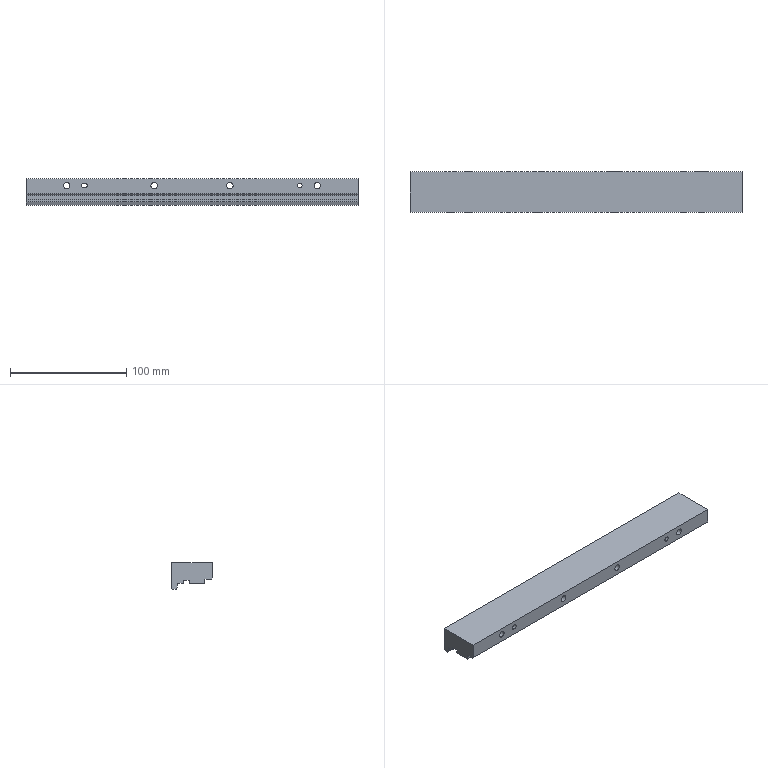Part | NX | 1 solid | 35 faces | box 285 x 35 x 22.9 mm | volume 168011 mm3 | plane 24 | cylinder 11 | commonest cylinder face diameters 5.5 x4 10 x4 4 x3
STEP:
#1=CARTESIAN_POINT('',(142.5,-17.5,-13.1));
#2=VERTEX_POINT('',#1);
#3=CARTESIAN_POINT('',(142.5,-16.5,-14.1));
#4=VERTEX_POINT('',#3);
#5=CARTESIAN_POINT('',(142.5,-17.5,-13.1));
#6=DIRECTION('',(0.,0.7071,-0.7071));
#7=VECTOR('',#6,1000.);
#8=LINE('',#5,#7);
#9=EDGE_CURVE('',#2,#4,#8,.T.);
#10=ORIENTED_EDGE('',*,*,#9,.T.);
#11=CARTESIAN_POINT('',(142.5,-11.14,-14.1));
#12=VERTEX_POINT('',#11);
#13=CARTESIAN_POINT('',(142.5,-17.5,-14.1));
#14=DIRECTION('',(0.,-1.,0.));
#15=VECTOR('',#14,1000.);
#16=LINE('',#13,#15);
#17=EDGE_CURVE('',#12,#4,#16,.T.);
#18=ORIENTED_EDGE('',*,*,#17,.F.);
#19=CARTESIAN_POINT('',(142.5,-11.14,-17.9));
#20=VERTEX_POINT('',#19);
#21=CARTESIAN_POINT('',(142.5,-11.14,-14.1));
#22=DIRECTION('',(0.,0.,1.));
#23=VECTOR('',#22,1000.);
#24=LINE('',#21,#23);
#25=EDGE_CURVE('',#20,#12,#24,.T.);
#26=ORIENTED_EDGE('',*,*,#25,.F.);
#27=CARTESIAN_POINT('',(142.5,2.3,-17.9));
#28=VERTEX_POINT('',#27);
#29=CARTESIAN_POINT('',(142.5,17.5,-17.9));
#30=DIRECTION('',(0.,-1.,0.));
#31=VECTOR('',#30,1000.);
#32=LINE('',#29,#31);
#33=EDGE_CURVE('',#28,#20,#32,.T.);
#34=ORIENTED_EDGE('',*,*,#33,.F.);
#35=CARTESIAN_POINT('',(142.5,2.3,-14.9));
#36=VERTEX_POINT('',#35);
#37=CARTESIAN_POINT('',(142.5,2.3,-17.9));
#38=DIRECTION('',(0.,0.,-1.));
#39=VECTOR('',#38,1000.);
#40=LINE('',#37,#39);
#41=EDGE_CURVE('',#36,#28,#40,.T.);
#42=ORIENTED_EDGE('',*,*,#41,.F.);
#43=CARTESIAN_POINT('',(142.5,7.3,-14.9));
#44=VERTEX_POINT('',#43);
#45=CARTESIAN_POINT('',(142.5,2.3,-14.9));
#46=DIRECTION('',(0.,-1.,0.));
#47=VECTOR('',#46,1000.);
#48=LINE('',#45,#47);
#49=EDGE_CURVE('',#44,#36,#48,.T.);
#50=ORIENTED_EDGE('',*,*,#49,.F.);
#51=CARTESIAN_POINT('',(142.5,7.3,-17.04));
#52=VERTEX_POINT('',#51);
#53=CARTESIAN_POINT('',(142.5,7.3,-14.9));
#54=DIRECTION('',(0.,0.,1.));
#55=VECTOR('',#54,1000.);
#56=LINE('',#53,#55);
#57=EDGE_CURVE('',#52,#44,#56,.T.);
#58=ORIENTED_EDGE('',*,*,#57,.F.);
#59=CARTESIAN_POINT('',(142.5,7.533,-17.54));
#60=VERTEX_POINT('',#59);
#61=CARTESIAN_POINT('',(142.5,7.3,-17.04));
#62=DIRECTION('',(0.,0.4226,-0.9063));
#63=VECTOR('',#62,1000.);
#64=LINE('',#61,#63);
#65=EDGE_CURVE('',#52,#60,#64,.T.);
#66=ORIENTED_EDGE('',*,*,#65,.T.);
#67=CARTESIAN_POINT('',(142.5,12.2,-17.54));
#68=VERTEX_POINT('',#67);
#69=CARTESIAN_POINT('',(142.5,7.3,-17.54));
#70=DIRECTION('',(0.,-1.,0.));
#71=VECTOR('',#70,1000.);
#72=LINE('',#69,#71);
#73=EDGE_CURVE('',#68,#60,#72,.T.);
#74=ORIENTED_EDGE('',*,*,#73,.F.);
#75=CARTESIAN_POINT('',(142.5,12.2,-19.9));
#76=VERTEX_POINT('',#75);
#77=CARTESIAN_POINT('',(142.5,12.2,-17.54));
#78=DIRECTION('',(0.,0.,1.));
#79=VECTOR('',#78,1000.);
#80=LINE('',#77,#79);
#81=EDGE_CURVE('',#76,#68,#80,.T.);
#82=ORIENTED_EDGE('',*,*,#81,.F.);
#83=CARTESIAN_POINT('',(142.5,13.599,-22.9));
#84=VERTEX_POINT('',#83);
#85=CARTESIAN_POINT('',(142.5,13.599,-22.9));
#86=DIRECTION('',(0.,0.4226,-0.9063));
#87=VECTOR('',#86,1000.);
#88=LINE('',#85,#87);
#89=EDGE_CURVE('',#76,#84,#88,.T.);
#90=ORIENTED_EDGE('',*,*,#89,.T.);
#91=CARTESIAN_POINT('',(142.5,16.5,-22.9));
#92=VERTEX_POINT('',#91);
#93=CARTESIAN_POINT('',(142.5,0.,-22.9));
#94=DIRECTION('',(0.,1.,0.));
#95=VECTOR('',#94,1000.);
#96=LINE('',#93,#95);
#97=EDGE_CURVE('',#84,#92,#96,.T.);
#98=ORIENTED_EDGE('',*,*,#97,.T.);
#99=CARTESIAN_POINT('',(142.5,17.5,-21.9));
#100=VERTEX_POINT('',#99);
#101=CARTESIAN_POINT('',(142.5,16.5,-22.9));
#102=DIRECTION('',(0.,0.7071,0.7071));
#103=VECTOR('',#102,1000.);
#104=LINE('',#101,#103);
#105=EDGE_CURVE('',#92,#100,#104,.T.);
#106=ORIENTED_EDGE('',*,*,#105,.T.);
#107=CARTESIAN_POINT('',(142.5,17.5,0.));
#108=VERTEX_POINT('',#107);
#109=CARTESIAN_POINT('',(142.5,17.5,-17.9));
#110=DIRECTION('',(0.,0.,1.));
#111=VECTOR('',#110,1000.);
#112=LINE('',#109,#111);
#113=EDGE_CURVE('',#100,#108,#112,.T.);
#114=ORIENTED_EDGE('',*,*,#113,.T.);
#115=CARTESIAN_POINT('',(142.5,-17.5,0.));
#116=VERTEX_POINT('',#115);
#117=CARTESIAN_POINT('',(142.5,17.5,0.));
#118=DIRECTION('',(0.,1.,0.));
#119=VECTOR('',#118,1000.);
#120=LINE('',#117,#119);
#121=EDGE_CURVE('',#116,#108,#120,.T.);
#122=ORIENTED_EDGE('',*,*,#121,.F.);
#123=CARTESIAN_POINT('',(142.5,-17.5,-17.9));
#124=DIRECTION('',(0.,0.,1.));
#125=VECTOR('',#124,1000.);
#126=LINE('',#123,#125);
#127=EDGE_CURVE('',#2,#116,#126,.T.);
#128=ORIENTED_EDGE('',*,*,#127,.F.);
#129=EDGE_LOOP('',(#10,#18,#26,#34,#42,#50,#58,#66,#74,#82,#90,#98,#106,#114,#122,#128));
#130=FACE_BOUND('',#129,.T.);
#131=CARTESIAN_POINT('',(142.5,17.5,-22.91));
#132=DIRECTION('',(-1.,0.,0.));
#133=DIRECTION('',(0.,0.,-1.));
#134=AXIS2_PLACEMENT_3D('',#131,#132,#133);
#135=PLANE('',#134);
#136=ADVANCED_FACE('',(#130),#135,.F.);
#137=ORIENTED_EDGE('',*,*,#65,.F.);
#138=CARTESIAN_POINT('',(-142.5,7.3,-17.04));
#139=VERTEX_POINT('',#138);
#140=CARTESIAN_POINT('',(-142.5,7.3,-17.04));
#141=DIRECTION('',(1.,0.,0.));
#142=VECTOR('',#141,1000.);
#143=LINE('',#140,#142);
#144=EDGE_CURVE('',#139,#52,#143,.T.);
#145=ORIENTED_EDGE('',*,*,#144,.F.);
#146=CARTESIAN_POINT('',(-142.5,7.533,-17.54));
#147=VERTEX_POINT('',#146);
#148=CARTESIAN_POINT('',(-142.5,7.3,-17.04));
#149=DIRECTION('',(0.,-0.4226,0.9063));
#150=VECTOR('',#149,1000.);
#151=LINE('',#148,#150);
#152=EDGE_CURVE('',#147,#139,#151,.T.);
#153=ORIENTED_EDGE('',*,*,#152,.F.);
#154=CARTESIAN_POINT('',(-142.5,7.533,-17.54));
#155=DIRECTION('',(-1.,0.,0.));
#156=VECTOR('',#155,1000.);
#157=LINE('',#154,#156);
#158=EDGE_CURVE('',#60,#147,#157,.T.);
#159=ORIENTED_EDGE('',*,*,#158,.F.);
#160=EDGE_LOOP('',(#137,#145,#153,#159));
#161=FACE_BOUND('',#160,.T.);
#162=CARTESIAN_POINT('',(-142.5,7.3,-17.04));
#163=DIRECTION('',(0.,0.9063,0.4226));
#164=DIRECTION('',(-1.,0.,0.));
#165=AXIS2_PLACEMENT_3D('',#162,#163,#164);
#166=PLANE('',#165);
#167=ADVANCED_FACE('',(#161),#166,.F.);
#168=ORIENTED_EDGE('',*,*,#144,.T.);
#169=ORIENTED_EDGE('',*,*,#57,.T.);
#170=CARTESIAN_POINT('',(-142.5,7.3,-14.9));
#171=VERTEX_POINT('',#170);
#172=CARTESIAN_POINT('',(-142.5,7.3,-14.9));
#173=DIRECTION('',(1.,0.,0.));
#174=VECTOR('',#173,1000.);
#175=LINE('',#172,#174);
#176=EDGE_CURVE('',#171,#44,#175,.T.);
#177=ORIENTED_EDGE('',*,*,#176,.F.);
#178=CARTESIAN_POINT('',(-142.5,7.3,-14.9));
#179=DIRECTION('',(0.,0.,1.));
#180=VECTOR('',#179,1000.);
#181=LINE('',#178,#180);
#182=EDGE_CURVE('',#139,#171,#181,.T.);
#183=ORIENTED_EDGE('',*,*,#182,.F.);
#184=EDGE_LOOP('',(#168,#169,#177,#183));
#185=FACE_BOUND('',#184,.T.);
#186=CARTESIAN_POINT('',(-142.5,7.3,-14.9));
#187=DIRECTION('',(0.,1.,0.));
#188=DIRECTION('',(0.,0.,1.));
#189=AXIS2_PLACEMENT_3D('',#186,#187,#188);
#190=PLANE('',#189);
#191=ADVANCED_FACE('',(#185),#190,.F.);
#192=CARTESIAN_POINT('',(-142.5,-11.14,-17.9));
#193=VERTEX_POINT('',#192);
#194=CARTESIAN_POINT('',(-142.5,-11.14,-17.9));
#195=DIRECTION('',(1.,0.,0.));
#196=VECTOR('',#195,1000.);
#197=LINE('',#194,#196);
#198=EDGE_CURVE('',#193,#20,#197,.T.);
#199=ORIENTED_EDGE('',*,*,#198,.T.);
#200=ORIENTED_EDGE('',*,*,#25,.T.);
#201=CARTESIAN_POINT('',(-142.5,-11.14,-14.1));
#202=VERTEX_POINT('',#201);
#203=CARTESIAN_POINT('',(-142.5,-11.14,-14.1));
#204=DIRECTION('',(1.,0.,0.));
#205=VECTOR('',#204,1000.);
#206=LINE('',#203,#205);
#207=EDGE_CURVE('',#202,#12,#206,.T.);
#208=ORIENTED_EDGE('',*,*,#207,.F.);
#209=CARTESIAN_POINT('',(-142.5,-11.14,-14.1));
#210=DIRECTION('',(0.,0.,1.));
#211=VECTOR('',#210,1000.);
#212=LINE('',#209,#211);
#213=EDGE_CURVE('',#193,#202,#212,.T.);
#214=ORIENTED_EDGE('',*,*,#213,.F.);
#215=EDGE_LOOP('',(#199,#200,#208,#214));
#216=FACE_BOUND('',#215,.T.);
#217=CARTESIAN_POINT('',(-142.5,-11.14,-14.1));
#218=DIRECTION('',(0.,1.,0.));
#219=DIRECTION('',(0.,0.,1.));
#220=AXIS2_PLACEMENT_3D('',#217,#218,#219);
#221=PLANE('',#220);
#222=ADVANCED_FACE('',(#216),#221,.F.);
#223=CARTESIAN_POINT('',(-142.5,2.3,-17.9));
#224=VERTEX_POINT('',#223);
#225=CARTESIAN_POINT('',(-142.5,2.3,-17.9));
#226=DIRECTION('',(1.,0.,0.));
#227=VECTOR('',#226,1000.);
#228=LINE('',#225,#227);
#229=EDGE_CURVE('',#224,#28,#228,.T.);
#230=ORIENTED_EDGE('',*,*,#229,.T.);
#231=ORIENTED_EDGE('',*,*,#33,.T.);
#232=ORIENTED_EDGE('',*,*,#198,.F.);
#233=CARTESIAN_POINT('',(-142.5,17.5,-17.9));
#234=DIRECTION('',(0.,-1.,0.));
#235=VECTOR('',#234,1000.);
#236=LINE('',#233,#235);
#237=EDGE_CURVE('',#224,#193,#236,.T.);
#238=ORIENTED_EDGE('',*,*,#237,.F.);
#239=EDGE_LOOP('',(#230,#231,#232,#238));
#240=FACE_BOUND('',#239,.T.);
#241=CARTESIAN_POINT('',(1442.5,17.5,-17.9));
#242=DIRECTION('',(0.,0.,1.));
#243=DIRECTION('',(-1.,0.,0.));
#244=AXIS2_PLACEMENT_3D('',#241,#242,#243);
#245=PLANE('',#244);
#246=ADVANCED_FACE('',(#240),#245,.F.);
#247=ORIENTED_EDGE('',*,*,#9,.F.);
#248=CARTESIAN_POINT('',(-142.5,-17.5,-13.1));
#249=VERTEX_POINT('',#248);
#250=CARTESIAN_POINT('',(1442.5,-17.5,-13.1));
#251=DIRECTION('',(1.,0.,0.));
#252=VECTOR('',#251,1000.);
#253=LINE('',#250,#252);
#254=EDGE_CURVE('',#249,#2,#253,.T.);
#255=ORIENTED_EDGE('',*,*,#254,.F.);
#256=CARTESIAN_POINT('',(-142.5,-16.5,-14.1));
#257=VERTEX_POINT('',#256);
#258=CARTESIAN_POINT('',(-142.5,-17.5,-13.1));
#259=DIRECTION('',(0.,-0.7071,0.7071));
#260=VECTOR('',#259,1000.);
#261=LINE('',#258,#260);
#262=EDGE_CURVE('',#257,#249,#261,.T.);
#263=ORIENTED_EDGE('',*,*,#262,.F.);
#264=CARTESIAN_POINT('',(-142.5,-16.5,-14.1));
#265=DIRECTION('',(-1.,0.,0.));
#266=VECTOR('',#265,1000.);
#267=LINE('',#264,#266);
#268=EDGE_CURVE('',#4,#257,#267,.T.);
#269=ORIENTED_EDGE('',*,*,#268,.F.);
#270=EDGE_LOOP('',(#247,#255,#263,#269));
#271=FACE_BOUND('',#270,.T.);
#272=CARTESIAN_POINT('',(1442.5,-17.5,-13.1));
#273=DIRECTION('',(0.,0.7071,0.7071));
#274=DIRECTION('',(-1.,0.,0.));
#275=AXIS2_PLACEMENT_3D('',#272,#273,#274);
#276=PLANE('',#275);
#277=ADVANCED_FACE('',(#271),#276,.F.);
#278=CARTESIAN_POINT('',(-92.,-17.5,-8.));
#279=VERTEX_POINT('',#278);
#280=CARTESIAN_POINT('',(-93.,-17.5,-8.));
#281=VERTEX_POINT('',#280);
#282=CARTESIAN_POINT('',(-93.,-17.5,-8.));
#283=DIRECTION('',(-1.,0.,0.));
#284=VECTOR('',#283,1000.);
#285=LINE('',#282,#284);
#286=EDGE_CURVE('',#279,#281,#285,.T.);
#287=ORIENTED_EDGE('',*,*,#286,.T.);
#288=CARTESIAN_POINT('',(-93.,-17.5,-4.));
#289=VERTEX_POINT('',#288);
#290=CARTESIAN_POINT('',(-93.,-17.5,-6.));
#291=DIRECTION('',(0.,1.,0.));
#292=DIRECTION('',(0.,0.,-1.));
#293=AXIS2_PLACEMENT_3D('',#290,#291,#292);
#294=CIRCLE('',#293,2.);
#295=EDGE_CURVE('',#281,#289,#294,.T.);
#296=ORIENTED_EDGE('',*,*,#295,.T.);
#297=CARTESIAN_POINT('',(-92.,-17.5,-4.));
#298=VERTEX_POINT('',#297);
#299=CARTESIAN_POINT('',(-93.,-17.5,-4.));
#300=DIRECTION('',(1.,0.,0.));
#301=VECTOR('',#300,1000.);
#302=LINE('',#299,#301);
#303=EDGE_CURVE('',#289,#298,#302,.T.);
#304=ORIENTED_EDGE('',*,*,#303,.T.);
#305=CARTESIAN_POINT('',(-92.,-17.5,-6.));
#306=DIRECTION('',(0.,1.,0.));
#307=DIRECTION('',(0.,0.,-1.));
#308=AXIS2_PLACEMENT_3D('',#305,#306,#307);
#309=CIRCLE('',#308,2.);
#310=EDGE_CURVE('',#298,#279,#309,.T.);
#311=ORIENTED_EDGE('',*,*,#310,.T.);
#312=EDGE_LOOP('',(#287,#296,#304,#311));
#313=FACE_BOUND('',#312,.T.);
#314=CARTESIAN_POINT('',(92.5,-17.5,-8.));
#315=VERTEX_POINT('',#314);
#316=CARTESIAN_POINT('',(92.5,-17.5,-6.));
#317=DIRECTION('',(0.,1.,0.));
#318=DIRECTION('',(0.,0.,-1.));
#319=AXIS2_PLACEMENT_3D('',#316,#317,#318);
#320=CIRCLE('',#319,2.);
#321=EDGE_CURVE('',#315,#315,#320,.T.);
#322=ORIENTED_EDGE('',*,*,#321,.T.);
#323=EDGE_LOOP('',(#322));
#324=FACE_BOUND('',#323,.T.);
#325=CARTESIAN_POINT('',(107.5,-17.5,-8.75));
#326=VERTEX_POINT('',#325);
#327=CARTESIAN_POINT('',(107.5,-17.5,-6.));
#328=DIRECTION('',(0.,1.,0.));
#329=DIRECTION('',(0.,0.,-1.));
#330=AXIS2_PLACEMENT_3D('',#327,#328,#329);
#331=CIRCLE('',#330,2.75);
#332=EDGE_CURVE('',#326,#326,#331,.T.);
#333=ORIENTED_EDGE('',*,*,#332,.T.);
#334=EDGE_LOOP('',(#333));
#335=FACE_BOUND('',#334,.T.);
#336=CARTESIAN_POINT('',(32.5,-17.5,-8.75));
#337=VERTEX_POINT('',#336);
#338=CARTESIAN_POINT('',(32.5,-17.5,-6.));
#339=DIRECTION('',(0.,1.,0.));
#340=DIRECTION('',(0.,0.,-1.));
#341=AXIS2_PLACEMENT_3D('',#338,#339,#340);
#342=CIRCLE('',#341,2.75);
#343=EDGE_CURVE('',#337,#337,#342,.T.);
#344=ORIENTED_EDGE('',*,*,#343,.T.);
#345=EDGE_LOOP('',(#344));
#346=FACE_BOUND('',#345,.T.);
#347=CARTESIAN_POINT('',(-32.5,-17.5,-8.75));
#348=VERTEX_POINT('',#347);
#349=CARTESIAN_POINT('',(-32.5,-17.5,-6.));
#350=DIRECTION('',(0.,1.,0.));
#351=DIRECTION('',(0.,0.,-1.));
#352=AXIS2_PLACEMENT_3D('',#349,#350,#351);
#353=CIRCLE('',#352,2.75);
#354=EDGE_CURVE('',#348,#348,#353,.T.);
#355=ORIENTED_EDGE('',*,*,#354,.T.);
#356=EDGE_LOOP('',(#355));
#357=FACE_BOUND('',#356,.T.);
#358=CARTESIAN_POINT('',(-107.5,-17.5,-8.75));
#359=VERTEX_POINT('',#358);
#360=CARTESIAN_POINT('',(-107.5,-17.5,-6.));
#361=DIRECTION('',(0.,1.,0.));
#362=DIRECTION('',(0.,0.,-1.));
#363=AXIS2_PLACEMENT_3D('',#360,#361,#362);
#364=CIRCLE('',#363,2.75);
#365=EDGE_CURVE('',#359,#359,#364,.T.);
#366=ORIENTED_EDGE('',*,*,#365,.T.);
#367=EDGE_LOOP('',(#366));
#368=FACE_BOUND('',#367,.T.);
#369=ORIENTED_EDGE('',*,*,#254,.T.);
#370=ORIENTED_EDGE('',*,*,#127,.T.);
#371=CARTESIAN_POINT('',(-142.5,-17.5,0.));
#372=VERTEX_POINT('',#371);
#373=CARTESIAN_POINT('',(1442.5,-17.5,0.));
#374=DIRECTION('',(1.,0.,0.));
#375=VECTOR('',#374,1000.);
#376=LINE('',#373,#375);
#377=EDGE_CURVE('',#372,#116,#376,.T.);
#378=ORIENTED_EDGE('',*,*,#377,.F.);
#379=CARTESIAN_POINT('',(-142.5,-17.5,0.));
#380=DIRECTION('',(0.,0.,1.));
#381=VECTOR('',#380,1000.);
#382=LINE('',#379,#381);
#383=EDGE_CURVE('',#249,#372,#382,.T.);
#384=ORIENTED_EDGE('',*,*,#383,.F.);
#385=EDGE_LOOP('',(#369,#370,#378,#384));
#386=FACE_BOUND('',#385,.T.);
#387=CARTESIAN_POINT('',(1442.5,-17.5,-17.9));
#388=DIRECTION('',(0.,1.,0.));
#389=DIRECTION('',(0.,0.,1.));
#390=AXIS2_PLACEMENT_3D('',#387,#388,#389);
#391=PLANE('',#390);
#392=ADVANCED_FACE('',(#313,#324,#335,#346,#357,#368,#386),#391,.F.);
#393=ORIENTED_EDGE('',*,*,#89,.F.);
#394=CARTESIAN_POINT('',(-142.5,12.2,-19.9));
#395=VERTEX_POINT('',#394);
#396=CARTESIAN_POINT('',(1442.5,12.2,-19.9));
#397=DIRECTION('',(1.,0.,0.));
#398=VECTOR('',#397,1000.);
#399=LINE('',#396,#398);
#400=EDGE_CURVE('',#395,#76,#399,.T.);
#401=ORIENTED_EDGE('',*,*,#400,.F.);
#402=CARTESIAN_POINT('',(-142.5,13.599,-22.9));
#403=VERTEX_POINT('',#402);
#404=CARTESIAN_POINT('',(-142.5,13.599,-22.9));
#405=DIRECTION('',(0.,-0.4226,0.9063));
#406=VECTOR('',#405,1000.);
#407=LINE('',#404,#406);
#408=EDGE_CURVE('',#403,#395,#407,.T.);
#409=ORIENTED_EDGE('',*,*,#408,.F.);
#410=CARTESIAN_POINT('',(-142.5,13.599,-22.9));
#411=DIRECTION('',(-1.,0.,0.));
#412=VECTOR('',#411,1000.);
#413=LINE('',#410,#412);
#414=EDGE_CURVE('',#84,#403,#413,.T.);
#415=ORIENTED_EDGE('',*,*,#414,.F.);
#416=EDGE_LOOP('',(#393,#401,#409,#415));
#417=FACE_BOUND('',#416,.T.);
#418=CARTESIAN_POINT('',(650.,13.599,-22.9));
#419=DIRECTION('',(0.,-0.9063,-0.4226));
#420=DIRECTION('',(-1.,0.,0.));
#421=AXIS2_PLACEMENT_3D('',#418,#419,#420);
#422=PLANE('',#421);
#423=ADVANCED_FACE('',(#417),#422,.T.);
#424=ORIENTED_EDGE('',*,*,#400,.T.);
#425=ORIENTED_EDGE('',*,*,#81,.T.);
#426=CARTESIAN_POINT('',(-142.5,12.2,-17.54));
#427=VERTEX_POINT('',#426);
#428=CARTESIAN_POINT('',(-142.5,12.2,-17.54));
#429=DIRECTION('',(1.,0.,0.));
#430=VECTOR('',#429,1000.);
#431=LINE('',#428,#430);
#432=EDGE_CURVE('',#427,#68,#431,.T.);
#433=ORIENTED_EDGE('',*,*,#432,.F.);
#434=CARTESIAN_POINT('',(-142.5,12.2,-17.54));
#435=DIRECTION('',(0.,0.,1.));
#436=VECTOR('',#435,1000.);
#437=LINE('',#434,#436);
#438=EDGE_CURVE('',#395,#427,#437,.T.);
#439=ORIENTED_EDGE('',*,*,#438,.F.);
#440=EDGE_LOOP('',(#424,#425,#433,#439));
#441=FACE_BOUND('',#440,.T.);
#442=CARTESIAN_POINT('',(-142.5,12.2,-17.54));
#443=DIRECTION('',(0.,1.,0.));
#444=DIRECTION('',(0.,0.,1.));
#445=AXIS2_PLACEMENT_3D('',#442,#443,#444);
#446=PLANE('',#445);
#447=ADVANCED_FACE('',(#441),#446,.F.);
#448=ORIENTED_EDGE('',*,*,#105,.F.);
#449=CARTESIAN_POINT('',(-142.5,16.5,-22.9));
#450=VERTEX_POINT('',#449);
#451=CARTESIAN_POINT('',(650.,16.5,-22.9));
#452=DIRECTION('',(1.,0.,0.));
#453=VECTOR('',#452,1000.);
#454=LINE('',#451,#453);
#455=EDGE_CURVE('',#450,#92,#454,.T.);
#456=ORIENTED_EDGE('',*,*,#455,.F.);
#457=CARTESIAN_POINT('',(-142.5,17.5,-21.9));
#458=VERTEX_POINT('',#457);
#459=CARTESIAN_POINT('',(-142.5,16.5,-22.9));
#460=DIRECTION('',(0.,-0.7071,-0.7071));
#461=VECTOR('',#460,1000.);
#462=LINE('',#459,#461);
#463=EDGE_CURVE('',#458,#450,#462,.T.);
#464=ORIENTED_EDGE('',*,*,#463,.F.);
#465=CARTESIAN_POINT('',(1442.5,17.5,-21.9));
#466=DIRECTION('',(-1.,0.,0.));
#467=VECTOR('',#466,1000.);
#468=LINE('',#465,#467);
#469=EDGE_CURVE('',#100,#458,#468,.T.);
#470=ORIENTED_EDGE('',*,*,#469,.F.);
#471=EDGE_LOOP('',(#448,#456,#464,#470));
#472=FACE_BOUND('',#471,.T.);
#473=CARTESIAN_POINT('',(650.,16.5,-22.9));
#474=DIRECTION('',(0.,-0.7071,0.7071));
#475=DIRECTION('',(-1.,0.,0.));
#476=AXIS2_PLACEMENT_3D('',#473,#474,#475);
#477=PLANE('',#476);
#478=ADVANCED_FACE('',(#472),#477,.F.);
#479=ORIENTED_EDGE('',*,*,#97,.F.);
#480=ORIENTED_EDGE('',*,*,#414,.T.);
#481=CARTESIAN_POINT('',(-142.5,17.5,-22.9));
#482=DIRECTION('',(0.,1.,0.));
#483=VECTOR('',#482,1000.);
#484=LINE('',#481,#483);
#485=EDGE_CURVE('',#403,#450,#484,.T.);
#486=ORIENTED_EDGE('',*,*,#485,.T.);
#487=ORIENTED_EDGE('',*,*,#455,.T.);
#488=EDGE_LOOP('',(#479,#480,#486,#487));
#489=FACE_BOUND('',#488,.T.);
#490=CARTESIAN_POINT('',(650.,0.,-22.9));
#491=DIRECTION('',(0.,0.,-1.));
#492=DIRECTION('',(1.,0.,0.));
#493=AXIS2_PLACEMENT_3D('',#490,#491,#492);
#494=PLANE('',#493);
#495=ADVANCED_FACE('',(#489),#494,.T.);
#496=CARTESIAN_POINT('',(-142.5,17.5,0.));
#497=VERTEX_POINT('',#496);
#498=CARTESIAN_POINT('',(-142.5,17.5,0.));
#499=DIRECTION('',(0.,0.,1.));
#500=VECTOR('',#499,1000.);
#501=LINE('',#498,#500);
#502=EDGE_CURVE('',#458,#497,#501,.T.);
#503=ORIENTED_EDGE('',*,*,#502,.F.);
#504=ORIENTED_EDGE('',*,*,#463,.T.);
#505=ORIENTED_EDGE('',*,*,#485,.F.);
#506=ORIENTED_EDGE('',*,*,#408,.T.);
#507=ORIENTED_EDGE('',*,*,#438,.T.);
#508=CARTESIAN_POINT('',(-142.5,7.3,-17.54));
#509=DIRECTION('',(0.,-1.,0.));
#510=VECTOR('',#509,1000.);
#511=LINE('',#508,#510);
#512=EDGE_CURVE('',#427,#147,#511,.T.);
#513=ORIENTED_EDGE('',*,*,#512,.T.);
#514=ORIENTED_EDGE('',*,*,#152,.T.);
#515=ORIENTED_EDGE('',*,*,#182,.T.);
#516=CARTESIAN_POINT('',(-142.5,2.3,-14.9));
#517=VERTEX_POINT('',#516);
#518=CARTESIAN_POINT('',(-142.5,2.3,-14.9));
#519=DIRECTION('',(0.,-1.,0.));
#520=VECTOR('',#519,1000.);
#521=LINE('',#518,#520);
#522=EDGE_CURVE('',#171,#517,#521,.T.);
#523=ORIENTED_EDGE('',*,*,#522,.T.);
#524=CARTESIAN_POINT('',(-142.5,2.3,-17.9));
#525=DIRECTION('',(0.,0.,-1.));
#526=VECTOR('',#525,1000.);
#527=LINE('',#524,#526);
#528=EDGE_CURVE('',#517,#224,#527,.T.);
#529=ORIENTED_EDGE('',*,*,#528,.T.);
#530=ORIENTED_EDGE('',*,*,#237,.T.);
#531=ORIENTED_EDGE('',*,*,#213,.T.);
#532=CARTESIAN_POINT('',(-142.5,-17.5,-14.1));
#533=DIRECTION('',(0.,-1.,0.));
#534=VECTOR('',#533,1000.);
#535=LINE('',#532,#534);
#536=EDGE_CURVE('',#202,#257,#535,.T.);
#537=ORIENTED_EDGE('',*,*,#536,.T.);
#538=ORIENTED_EDGE('',*,*,#262,.T.);
#539=ORIENTED_EDGE('',*,*,#383,.T.);
#540=CARTESIAN_POINT('',(-142.5,17.5,0.));
#541=DIRECTION('',(0.,-1.,0.));
#542=VECTOR('',#541,1000.);
#543=LINE('',#540,#542);
#544=EDGE_CURVE('',#497,#372,#543,.T.);
#545=ORIENTED_EDGE('',*,*,#544,.F.);
#546=EDGE_LOOP('',(#503,#504,#505,#506,#507,#513,#514,#515,#523,#529,#530,#531,#537,#538,#539,#545));
#547=FACE_BOUND('',#546,.T.);
#548=CARTESIAN_POINT('',(-142.5,17.5,0.));
#549=DIRECTION('',(1.,0.,0.));
#550=DIRECTION('',(0.,0.,1.));
#551=AXIS2_PLACEMENT_3D('',#548,#549,#550);
#552=PLANE('',#551);
#553=ADVANCED_FACE('',(#547),#552,.F.);
#554=CARTESIAN_POINT('',(-93.,17.5,-8.));
#555=VERTEX_POINT('',#554);
#556=CARTESIAN_POINT('',(-93.,17.5,-4.));
#557=VERTEX_POINT('',#556);
#558=CARTESIAN_POINT('',(-93.,17.5,-6.));
#559=DIRECTION('',(0.,1.,0.));
#560=DIRECTION('',(0.,0.,-1.));
#561=AXIS2_PLACEMENT_3D('',#558,#559,#560);
#562=CIRCLE('',#561,2.);
#563=EDGE_CURVE('',#555,#557,#562,.T.);
#564=ORIENTED_EDGE('',*,*,#563,.F.);
#565=CARTESIAN_POINT('',(-92.,17.5,-8.));
#566=VERTEX_POINT('',#565);
#567=CARTESIAN_POINT('',(-93.,17.5,-8.));
#568=DIRECTION('',(-1.,0.,0.));
#569=VECTOR('',#568,1000.);
#570=LINE('',#567,#569);
#571=EDGE_CURVE('',#566,#555,#570,.T.);
#572=ORIENTED_EDGE('',*,*,#571,.F.);
#573=CARTESIAN_POINT('',(-92.,17.5,-4.));
#574=VERTEX_POINT('',#573);
#575=CARTESIAN_POINT('',(-92.,17.5,-6.));
#576=DIRECTION('',(0.,1.,0.));
#577=DIRECTION('',(0.,0.,-1.));
#578=AXIS2_PLACEMENT_3D('',#575,#576,#577);
#579=CIRCLE('',#578,2.);
#580=EDGE_CURVE('',#574,#566,#579,.T.);
#581=ORIENTED_EDGE('',*,*,#580,.F.);
#582=CARTESIAN_POINT('',(-93.,17.5,-4.));
#583=DIRECTION('',(1.,0.,0.));
#584=VECTOR('',#583,1000.);
#585=LINE('',#582,#584);
#586=EDGE_CURVE('',#557,#574,#585,.T.);
#587=ORIENTED_EDGE('',*,*,#586,.F.);
#588=EDGE_LOOP('',(#564,#572,#581,#587));
#589=FACE_BOUND('',#588,.T.);
#590=CARTESIAN_POINT('',(92.5,17.5,-8.));
#591=VERTEX_POINT('',#590);
#592=CARTESIAN_POINT('',(92.5,17.5,-6.));
#593=DIRECTION('',(0.,1.,0.));
#594=DIRECTION('',(0.,0.,-1.));
#595=AXIS2_PLACEMENT_3D('',#592,#593,#594);
#596=CIRCLE('',#595,2.);
#597=EDGE_CURVE('',#591,#591,#596,.T.);
#598=ORIENTED_EDGE('',*,*,#597,.F.);
#599=EDGE_LOOP('',(#598));
#600=FACE_BOUND('',#599,.T.);
#601=CARTESIAN_POINT('',(107.5,17.5,-11.));
#602=VERTEX_POINT('',#601);
#603=CARTESIAN_POINT('',(107.5,17.5,-6.));
#604=DIRECTION('',(0.,1.,0.));
#605=DIRECTION('',(0.,0.,-1.));
#606=AXIS2_PLACEMENT_3D('',#603,#604,#605);
#607=CIRCLE('',#606,5.);
#608=EDGE_CURVE('',#602,#602,#607,.T.);
#609=ORIENTED_EDGE('',*,*,#608,.F.);
#610=EDGE_LOOP('',(#609));
#611=FACE_BOUND('',#610,.T.);
#612=CARTESIAN_POINT('',(32.5,17.5,-11.));
#613=VERTEX_POINT('',#612);
#614=CARTESIAN_POINT('',(32.5,17.5,-6.));
#615=DIRECTION('',(0.,1.,0.));
#616=DIRECTION('',(0.,0.,-1.));
#617=AXIS2_PLACEMENT_3D('',#614,#615,#616);
#618=CIRCLE('',#617,5.);
#619=EDGE_CURVE('',#613,#613,#618,.T.);
#620=ORIENTED_EDGE('',*,*,#619,.F.);
#621=EDGE_LOOP('',(#620));
#622=FACE_BOUND('',#621,.T.);
#623=CARTESIAN_POINT('',(-32.5,17.5,-11.));
#624=VERTEX_POINT('',#623);
#625=CARTESIAN_POINT('',(-32.5,17.5,-6.));
#626=DIRECTION('',(0.,1.,0.));
#627=DIRECTION('',(0.,0.,-1.));
#628=AXIS2_PLACEMENT_3D('',#625,#626,#627);
#629=CIRCLE('',#628,5.);
#630=EDGE_CURVE('',#624,#624,#629,.T.);
#631=ORIENTED_EDGE('',*,*,#630,.F.);
#632=EDGE_LOOP('',(#631));
#633=FACE_BOUND('',#632,.T.);
#634=CARTESIAN_POINT('',(-107.5,17.5,-11.));
#635=VERTEX_POINT('',#634);
#636=CARTESIAN_POINT('',(-107.5,17.5,-6.));
#637=DIRECTION('',(0.,1.,0.));
#638=DIRECTION('',(0.,0.,-1.));
#639=AXIS2_PLACEMENT_3D('',#636,#637,#638);
#640=CIRCLE('',#639,5.);
#641=EDGE_CURVE('',#635,#635,#640,.T.);
#642=ORIENTED_EDGE('',*,*,#641,.F.);
#643=EDGE_LOOP('',(#642));
#644=FACE_BOUND('',#643,.T.);
#645=ORIENTED_EDGE('',*,*,#113,.F.);
#646=ORIENTED_EDGE('',*,*,#469,.T.);
#647=ORIENTED_EDGE('',*,*,#502,.T.);
#648=CARTESIAN_POINT('',(1442.5,17.5,0.));
#649=DIRECTION('',(1.,0.,0.));
#650=VECTOR('',#649,1000.);
#651=LINE('',#648,#650);
#652=EDGE_CURVE('',#497,#108,#651,.T.);
#653=ORIENTED_EDGE('',*,*,#652,.T.);
#654=EDGE_LOOP('',(#645,#646,#647,#653));
#655=FACE_BOUND('',#654,.T.);
#656=CARTESIAN_POINT('',(1442.5,17.5,-17.9));
#657=DIRECTION('',(0.,1.,0.));
#658=DIRECTION('',(0.,0.,1.));
#659=AXIS2_PLACEMENT_3D('',#656,#657,#658);
#660=PLANE('',#659);
#661=ADVANCED_FACE('',(#589,#600,#611,#622,#633,#644,#655),#660,.T.);
#662=ORIENTED_EDGE('',*,*,#207,.T.);
#663=ORIENTED_EDGE('',*,*,#17,.T.);
#664=ORIENTED_EDGE('',*,*,#268,.T.);
#665=ORIENTED_EDGE('',*,*,#536,.F.);
#666=EDGE_LOOP('',(#662,#663,#664,#665));
#667=FACE_BOUND('',#666,.T.);
#668=CARTESIAN_POINT('',(-142.5,-17.5,-14.1));
#669=DIRECTION('',(0.,0.,1.));
#670=DIRECTION('',(-1.,0.,0.));
#671=AXIS2_PLACEMENT_3D('',#668,#669,#670);
#672=PLANE('',#671);
#673=ADVANCED_FACE('',(#667),#672,.F.);
#674=ORIENTED_EDGE('',*,*,#432,.T.);
#675=ORIENTED_EDGE('',*,*,#73,.T.);
#676=ORIENTED_EDGE('',*,*,#158,.T.);
#677=ORIENTED_EDGE('',*,*,#512,.F.);
#678=EDGE_LOOP('',(#674,#675,#676,#677));
#679=FACE_BOUND('',#678,.T.);
#680=CARTESIAN_POINT('',(-142.5,7.3,-17.54));
#681=DIRECTION('',(0.,0.,1.));
#682=DIRECTION('',(-1.,0.,0.));
#683=AXIS2_PLACEMENT_3D('',#680,#681,#682);
#684=PLANE('',#683);
#685=ADVANCED_FACE('',(#679),#684,.F.);
#686=ORIENTED_EDGE('',*,*,#176,.T.);
#687=ORIENTED_EDGE('',*,*,#49,.T.);
#688=CARTESIAN_POINT('',(-142.5,2.3,-14.9));
#689=DIRECTION('',(1.,0.,0.));
#690=VECTOR('',#689,1000.);
#691=LINE('',#688,#690);
#692=EDGE_CURVE('',#517,#36,#691,.T.);
#693=ORIENTED_EDGE('',*,*,#692,.F.);
#694=ORIENTED_EDGE('',*,*,#522,.F.);
#695=EDGE_LOOP('',(#686,#687,#693,#694));
#696=FACE_BOUND('',#695,.T.);
#697=CARTESIAN_POINT('',(-142.5,2.3,-14.9));
#698=DIRECTION('',(0.,0.,1.));
#699=DIRECTION('',(-1.,0.,0.));
#700=AXIS2_PLACEMENT_3D('',#697,#698,#699);
#701=PLANE('',#700);
#702=ADVANCED_FACE('',(#696),#701,.F.);
#703=ORIENTED_EDGE('',*,*,#692,.T.);
#704=ORIENTED_EDGE('',*,*,#41,.T.);
#705=ORIENTED_EDGE('',*,*,#229,.F.);
#706=ORIENTED_EDGE('',*,*,#528,.F.);
#707=EDGE_LOOP('',(#703,#704,#705,#706));
#708=FACE_BOUND('',#707,.T.);
#709=CARTESIAN_POINT('',(-142.5,2.3,-17.9));
#710=DIRECTION('',(0.,-1.,0.));
#711=DIRECTION('',(0.,0.,-1.));
#712=AXIS2_PLACEMENT_3D('',#709,#710,#711);
#713=PLANE('',#712);
#714=ADVANCED_FACE('',(#708),#713,.F.);
#715=ORIENTED_EDGE('',*,*,#377,.T.);
#716=ORIENTED_EDGE('',*,*,#121,.T.);
#717=ORIENTED_EDGE('',*,*,#652,.F.);
#718=ORIENTED_EDGE('',*,*,#544,.T.);
#719=EDGE_LOOP('',(#715,#716,#717,#718));
#720=FACE_BOUND('',#719,.T.);
#721=CARTESIAN_POINT('',(1442.5,17.5,0.));
#722=DIRECTION('',(0.,0.,-1.));
#723=DIRECTION('',(1.,0.,0.));
#724=AXIS2_PLACEMENT_3D('',#721,#722,#723);
#725=PLANE('',#724);
#726=ADVANCED_FACE('',(#720),#725,.F.);
#727=ORIENTED_EDGE('',*,*,#365,.F.);
#728=EDGE_LOOP('',(#727));
#729=FACE_BOUND('',#728,.T.);
#730=CARTESIAN_POINT('',(-107.5,12.1,-8.75));
#731=VERTEX_POINT('',#730);
#732=CARTESIAN_POINT('',(-107.5,12.1,-6.));
#733=DIRECTION('',(0.,1.,0.));
#734=DIRECTION('',(0.,0.,-1.));
#735=AXIS2_PLACEMENT_3D('',#732,#733,#734);
#736=CIRCLE('',#735,2.75);
#737=EDGE_CURVE('',#731,#731,#736,.T.);
#738=ORIENTED_EDGE('',*,*,#737,.T.);
#739=EDGE_LOOP('',(#738));
#740=FACE_BOUND('',#739,.T.);
#741=CARTESIAN_POINT('',(-107.5,17.5,-6.));
#742=DIRECTION('',(0.,1.,0.));
#743=DIRECTION('',(0.,0.,1.));
#744=AXIS2_PLACEMENT_3D('',#741,#742,#743);
#745=CYLINDRICAL_SURFACE('',#744,2.75);
#746=ADVANCED_FACE('',(#729,#740),#745,.F.);
#747=ORIENTED_EDGE('',*,*,#737,.F.);
#748=EDGE_LOOP('',(#747));
#749=FACE_BOUND('',#748,.T.);
#750=CARTESIAN_POINT('',(-107.5,12.1,-11.));
#751=VERTEX_POINT('',#750);
#752=CARTESIAN_POINT('',(-107.5,12.1,-6.));
#753=DIRECTION('',(0.,1.,0.));
#754=DIRECTION('',(0.,0.,-1.));
#755=AXIS2_PLACEMENT_3D('',#752,#753,#754);
#756=CIRCLE('',#755,5.);
#757=EDGE_CURVE('',#751,#751,#756,.T.);
#758=ORIENTED_EDGE('',*,*,#757,.T.);
#759=EDGE_LOOP('',(#758));
#760=FACE_BOUND('',#759,.T.);
#761=CARTESIAN_POINT('',(-110.25,12.1,-6.));
#762=DIRECTION('',(0.,-1.,0.));
#763=DIRECTION('',(0.,0.,-1.));
#764=AXIS2_PLACEMENT_3D('',#761,#762,#763);
#765=PLANE('',#764);
#766=ADVANCED_FACE('',(#749,#760),#765,.F.);
#767=ORIENTED_EDGE('',*,*,#757,.F.);
#768=EDGE_LOOP('',(#767));
#769=FACE_BOUND('',#768,.T.);
#770=ORIENTED_EDGE('',*,*,#641,.T.);
#771=EDGE_LOOP('',(#770));
#772=FACE_BOUND('',#771,.T.);
#773=CARTESIAN_POINT('',(-107.5,17.5,-6.));
#774=DIRECTION('',(0.,1.,0.));
#775=DIRECTION('',(0.,0.,1.));
#776=AXIS2_PLACEMENT_3D('',#773,#774,#775);
#777=CYLINDRICAL_SURFACE('',#776,5.);
#778=ADVANCED_FACE('',(#769,#772),#777,.F.);
#779=ORIENTED_EDGE('',*,*,#354,.F.);
#780=EDGE_LOOP('',(#779));
#781=FACE_BOUND('',#780,.T.);
#782=CARTESIAN_POINT('',(-32.5,12.1,-8.75));
#783=VERTEX_POINT('',#782);
#784=CARTESIAN_POINT('',(-32.5,12.1,-6.));
#785=DIRECTION('',(0.,1.,0.));
#786=DIRECTION('',(0.,0.,-1.));
#787=AXIS2_PLACEMENT_3D('',#784,#785,#786);
#788=CIRCLE('',#787,2.75);
#789=EDGE_CURVE('',#783,#783,#788,.T.);
#790=ORIENTED_EDGE('',*,*,#789,.T.);
#791=EDGE_LOOP('',(#790));
#792=FACE_BOUND('',#791,.T.);
#793=CARTESIAN_POINT('',(-32.5,17.5,-6.));
#794=DIRECTION('',(0.,1.,0.));
#795=DIRECTION('',(0.,0.,1.));
#796=AXIS2_PLACEMENT_3D('',#793,#794,#795);
#797=CYLINDRICAL_SURFACE('',#796,2.75);
#798=ADVANCED_FACE('',(#781,#792),#797,.F.);
#799=ORIENTED_EDGE('',*,*,#789,.F.);
#800=EDGE_LOOP('',(#799));
#801=FACE_BOUND('',#800,.T.);
#802=CARTESIAN_POINT('',(-32.5,12.1,-11.));
#803=VERTEX_POINT('',#802);
#804=CARTESIAN_POINT('',(-32.5,12.1,-6.));
#805=DIRECTION('',(0.,1.,0.));
#806=DIRECTION('',(0.,0.,-1.));
#807=AXIS2_PLACEMENT_3D('',#804,#805,#806);
#808=CIRCLE('',#807,5.);
#809=EDGE_CURVE('',#803,#803,#808,.T.);
#810=ORIENTED_EDGE('',*,*,#809,.T.);
#811=EDGE_LOOP('',(#810));
#812=FACE_BOUND('',#811,.T.);
#813=CARTESIAN_POINT('',(-35.25,12.1,-6.));
#814=DIRECTION('',(0.,-1.,0.));
#815=DIRECTION('',(0.,0.,-1.));
#816=AXIS2_PLACEMENT_3D('',#813,#814,#815);
#817=PLANE('',#816);
#818=ADVANCED_FACE('',(#801,#812),#817,.F.);
#819=ORIENTED_EDGE('',*,*,#809,.F.);
#820=EDGE_LOOP('',(#819));
#821=FACE_BOUND('',#820,.T.);
#822=ORIENTED_EDGE('',*,*,#630,.T.);
#823=EDGE_LOOP('',(#822));
#824=FACE_BOUND('',#823,.T.);
#825=CARTESIAN_POINT('',(-32.5,17.5,-6.));
#826=DIRECTION('',(0.,1.,0.));
#827=DIRECTION('',(0.,0.,1.));
#828=AXIS2_PLACEMENT_3D('',#825,#826,#827);
#829=CYLINDRICAL_SURFACE('',#828,5.);
#830=ADVANCED_FACE('',(#821,#824),#829,.F.);
#831=ORIENTED_EDGE('',*,*,#343,.F.);
#832=EDGE_LOOP('',(#831));
#833=FACE_BOUND('',#832,.T.);
#834=CARTESIAN_POINT('',(32.5,12.1,-8.75));
#835=VERTEX_POINT('',#834);
#836=CARTESIAN_POINT('',(32.5,12.1,-6.));
#837=DIRECTION('',(0.,1.,0.));
#838=DIRECTION('',(0.,0.,-1.));
#839=AXIS2_PLACEMENT_3D('',#836,#837,#838);
#840=CIRCLE('',#839,2.75);
#841=EDGE_CURVE('',#835,#835,#840,.T.);
#842=ORIENTED_EDGE('',*,*,#841,.T.);
#843=EDGE_LOOP('',(#842));
#844=FACE_BOUND('',#843,.T.);
#845=CARTESIAN_POINT('',(32.5,17.5,-6.));
#846=DIRECTION('',(0.,1.,0.));
#847=DIRECTION('',(0.,0.,1.));
#848=AXIS2_PLACEMENT_3D('',#845,#846,#847);
#849=CYLINDRICAL_SURFACE('',#848,2.75);
#850=ADVANCED_FACE('',(#833,#844),#849,.F.);
#851=ORIENTED_EDGE('',*,*,#841,.F.);
#852=EDGE_LOOP('',(#851));
#853=FACE_BOUND('',#852,.T.);
#854=CARTESIAN_POINT('',(32.5,12.1,-11.));
#855=VERTEX_POINT('',#854);
#856=CARTESIAN_POINT('',(32.5,12.1,-6.));
#857=DIRECTION('',(0.,1.,0.));
#858=DIRECTION('',(0.,0.,-1.));
#859=AXIS2_PLACEMENT_3D('',#856,#857,#858);
#860=CIRCLE('',#859,5.);
#861=EDGE_CURVE('',#855,#855,#860,.T.);
#862=ORIENTED_EDGE('',*,*,#861,.T.);
#863=EDGE_LOOP('',(#862));
#864=FACE_BOUND('',#863,.T.);
#865=CARTESIAN_POINT('',(29.75,12.1,-6.));
#866=DIRECTION('',(0.,-1.,0.));
#867=DIRECTION('',(0.,0.,-1.));
#868=AXIS2_PLACEMENT_3D('',#865,#866,#867);
#869=PLANE('',#868);
#870=ADVANCED_FACE('',(#853,#864),#869,.F.);
#871=ORIENTED_EDGE('',*,*,#861,.F.);
#872=EDGE_LOOP('',(#871));
#873=FACE_BOUND('',#872,.T.);
#874=ORIENTED_EDGE('',*,*,#619,.T.);
#875=EDGE_LOOP('',(#874));
#876=FACE_BOUND('',#875,.T.);
#877=CARTESIAN_POINT('',(32.5,17.5,-6.));
#878=DIRECTION('',(0.,1.,0.));
#879=DIRECTION('',(0.,0.,1.));
#880=AXIS2_PLACEMENT_3D('',#877,#878,#879);
#881=CYLINDRICAL_SURFACE('',#880,5.);
#882=ADVANCED_FACE('',(#873,#876),#881,.F.);
#883=ORIENTED_EDGE('',*,*,#332,.F.);
#884=EDGE_LOOP('',(#883));
#885=FACE_BOUND('',#884,.T.);
#886=CARTESIAN_POINT('',(107.5,12.1,-8.75));
#887=VERTEX_POINT('',#886);
#888=CARTESIAN_POINT('',(107.5,12.1,-6.));
#889=DIRECTION('',(0.,1.,0.));
#890=DIRECTION('',(0.,0.,-1.));
#891=AXIS2_PLACEMENT_3D('',#888,#889,#890);
#892=CIRCLE('',#891,2.75);
#893=EDGE_CURVE('',#887,#887,#892,.T.);
#894=ORIENTED_EDGE('',*,*,#893,.T.);
#895=EDGE_LOOP('',(#894));
#896=FACE_BOUND('',#895,.T.);
#897=CARTESIAN_POINT('',(107.5,17.5,-6.));
#898=DIRECTION('',(0.,1.,0.));
#899=DIRECTION('',(0.,0.,1.));
#900=AXIS2_PLACEMENT_3D('',#897,#898,#899);
#901=CYLINDRICAL_SURFACE('',#900,2.75);
#902=ADVANCED_FACE('',(#885,#896),#901,.F.);
#903=ORIENTED_EDGE('',*,*,#893,.F.);
#904=EDGE_LOOP('',(#903));
#905=FACE_BOUND('',#904,.T.);
#906=CARTESIAN_POINT('',(107.5,12.1,-11.));
#907=VERTEX_POINT('',#906);
#908=CARTESIAN_POINT('',(107.5,12.1,-6.));
#909=DIRECTION('',(0.,1.,0.));
#910=DIRECTION('',(0.,0.,-1.));
#911=AXIS2_PLACEMENT_3D('',#908,#909,#910);
#912=CIRCLE('',#911,5.);
#913=EDGE_CURVE('',#907,#907,#912,.T.);
#914=ORIENTED_EDGE('',*,*,#913,.T.);
#915=EDGE_LOOP('',(#914));
#916=FACE_BOUND('',#915,.T.);
#917=CARTESIAN_POINT('',(104.75,12.1,-6.));
#918=DIRECTION('',(0.,-1.,0.));
#919=DIRECTION('',(0.,0.,-1.));
#920=AXIS2_PLACEMENT_3D('',#917,#918,#919);
#921=PLANE('',#920);
#922=ADVANCED_FACE('',(#905,#916),#921,.F.);
#923=ORIENTED_EDGE('',*,*,#913,.F.);
#924=EDGE_LOOP('',(#923));
#925=FACE_BOUND('',#924,.T.);
#926=ORIENTED_EDGE('',*,*,#608,.T.);
#927=EDGE_LOOP('',(#926));
#928=FACE_BOUND('',#927,.T.);
#929=CARTESIAN_POINT('',(107.5,17.5,-6.));
#930=DIRECTION('',(0.,1.,0.));
#931=DIRECTION('',(0.,0.,1.));
#932=AXIS2_PLACEMENT_3D('',#929,#930,#931);
#933=CYLINDRICAL_SURFACE('',#932,5.);
#934=ADVANCED_FACE('',(#925,#928),#933,.F.);
#935=ORIENTED_EDGE('',*,*,#321,.F.);
#936=EDGE_LOOP('',(#935));
#937=FACE_BOUND('',#936,.T.);
#938=ORIENTED_EDGE('',*,*,#597,.T.);
#939=EDGE_LOOP('',(#938));
#940=FACE_BOUND('',#939,.T.);
#941=CARTESIAN_POINT('',(92.5,-17.5,-6.));
#942=DIRECTION('',(0.,1.,0.));
#943=DIRECTION('',(0.,0.,1.));
#944=AXIS2_PLACEMENT_3D('',#941,#942,#943);
#945=CYLINDRICAL_SURFACE('',#944,2.);
#946=ADVANCED_FACE('',(#937,#940),#945,.F.);
#947=ORIENTED_EDGE('',*,*,#563,.T.);
#948=CARTESIAN_POINT('',(-93.,-17.5,-4.));
#949=DIRECTION('',(0.,1.,0.));
#950=VECTOR('',#949,1000.);
#951=LINE('',#948,#950);
#952=EDGE_CURVE('',#289,#557,#951,.T.);
#953=ORIENTED_EDGE('',*,*,#952,.F.);
#954=ORIENTED_EDGE('',*,*,#295,.F.);
#955=CARTESIAN_POINT('',(-93.,-17.5,-8.));
#956=DIRECTION('',(0.,1.,0.));
#957=VECTOR('',#956,1000.);
#958=LINE('',#955,#957);
#959=EDGE_CURVE('',#281,#555,#958,.T.);
#960=ORIENTED_EDGE('',*,*,#959,.T.);
#961=EDGE_LOOP('',(#947,#953,#954,#960));
#962=FACE_BOUND('',#961,.T.);
#963=CARTESIAN_POINT('',(-93.,-17.5,-6.));
#964=DIRECTION('',(0.,1.,0.));
#965=DIRECTION('',(0.,0.,1.));
#966=AXIS2_PLACEMENT_3D('',#963,#964,#965);
#967=CYLINDRICAL_SURFACE('',#966,2.);
#968=ADVANCED_FACE('',(#962),#967,.F.);
#969=ORIENTED_EDGE('',*,*,#571,.T.);
#970=ORIENTED_EDGE('',*,*,#959,.F.);
#971=ORIENTED_EDGE('',*,*,#286,.F.);
#972=CARTESIAN_POINT('',(-92.,-17.5,-8.));
#973=DIRECTION('',(0.,1.,0.));
#974=VECTOR('',#973,1000.);
#975=LINE('',#972,#974);
#976=EDGE_CURVE('',#279,#566,#975,.T.);
#977=ORIENTED_EDGE('',*,*,#976,.T.);
#978=EDGE_LOOP('',(#969,#970,#971,#977));
#979=FACE_BOUND('',#978,.T.);
#980=CARTESIAN_POINT('',(-93.,-17.5,-8.));
#981=DIRECTION('',(0.,0.,-1.));
#982=DIRECTION('',(1.,0.,0.));
#983=AXIS2_PLACEMENT_3D('',#980,#981,#982);
#984=PLANE('',#983);
#985=ADVANCED_FACE('',(#979),#984,.F.);
#986=ORIENTED_EDGE('',*,*,#580,.T.);
#987=ORIENTED_EDGE('',*,*,#976,.F.);
#988=ORIENTED_EDGE('',*,*,#310,.F.);
#989=CARTESIAN_POINT('',(-92.,-17.5,-4.));
#990=DIRECTION('',(0.,1.,0.));
#991=VECTOR('',#990,1000.);
#992=LINE('',#989,#991);
#993=EDGE_CURVE('',#298,#574,#992,.T.);
#994=ORIENTED_EDGE('',*,*,#993,.T.);
#995=EDGE_LOOP('',(#986,#987,#988,#994));
#996=FACE_BOUND('',#995,.T.);
#997=CARTESIAN_POINT('',(-92.,-17.5,-6.));
#998=DIRECTION('',(0.,1.,0.));
#999=DIRECTION('',(0.,0.,1.));
#1000=AXIS2_PLACEMENT_3D('',#997,#998,#999);
#1001=CYLINDRICAL_SURFACE('',#1000,2.);
#1002=ADVANCED_FACE('',(#996),#1001,.F.);
#1003=ORIENTED_EDGE('',*,*,#586,.T.);
#1004=ORIENTED_EDGE('',*,*,#993,.F.);
#1005=ORIENTED_EDGE('',*,*,#303,.F.);
#1006=ORIENTED_EDGE('',*,*,#952,.T.);
#1007=EDGE_LOOP('',(#1003,#1004,#1005,#1006));
#1008=FACE_BOUND('',#1007,.T.);
#1009=CARTESIAN_POINT('',(-93.,-17.5,-4.));
#1010=DIRECTION('',(0.,0.,1.));
#1011=DIRECTION('',(-1.,0.,0.));
#1012=AXIS2_PLACEMENT_3D('',#1009,#1010,#1011);
#1013=PLANE('',#1012);
#1014=ADVANCED_FACE('',(#1008),#1013,.F.);
#1015=CLOSED_SHELL('',(#136,#167,#191,#222,#246,#277,#392,#423,#447,#478,#495,#553,#661,#673,#685,#702,#714,#726,#746,#766,#778,#798,#818,#830,#850,#870,#882,#902,#922,#934,#946,#968,#985,#1002,#1014));
#1016=MANIFOLD_SOLID_BREP('',#1015);
#1017=(LENGTH_UNIT()NAMED_UNIT(*)SI_UNIT(.MILLI.,.METRE.));
#1018=UNCERTAINTY_MEASURE_WITH_UNIT(LENGTH_MEASURE(0.00001),#1017,'','');
#1019=(NAMED_UNIT(*)PLANE_ANGLE_UNIT()SI_UNIT($,.RADIAN.));
#1020=(NAMED_UNIT(*)SI_UNIT($,.STERADIAN.)SOLID_ANGLE_UNIT());
#1021=(GEOMETRIC_REPRESENTATION_CONTEXT(3)GLOBAL_UNCERTAINTY_ASSIGNED_CONTEXT((#1018))GLOBAL_UNIT_ASSIGNED_CONTEXT((#1017,#1019,#1020))REPRESENTATION_CONTEXT('',''));
#1022=ADVANCED_BREP_SHAPE_REPRESENTATION('',(#1016),#1021);